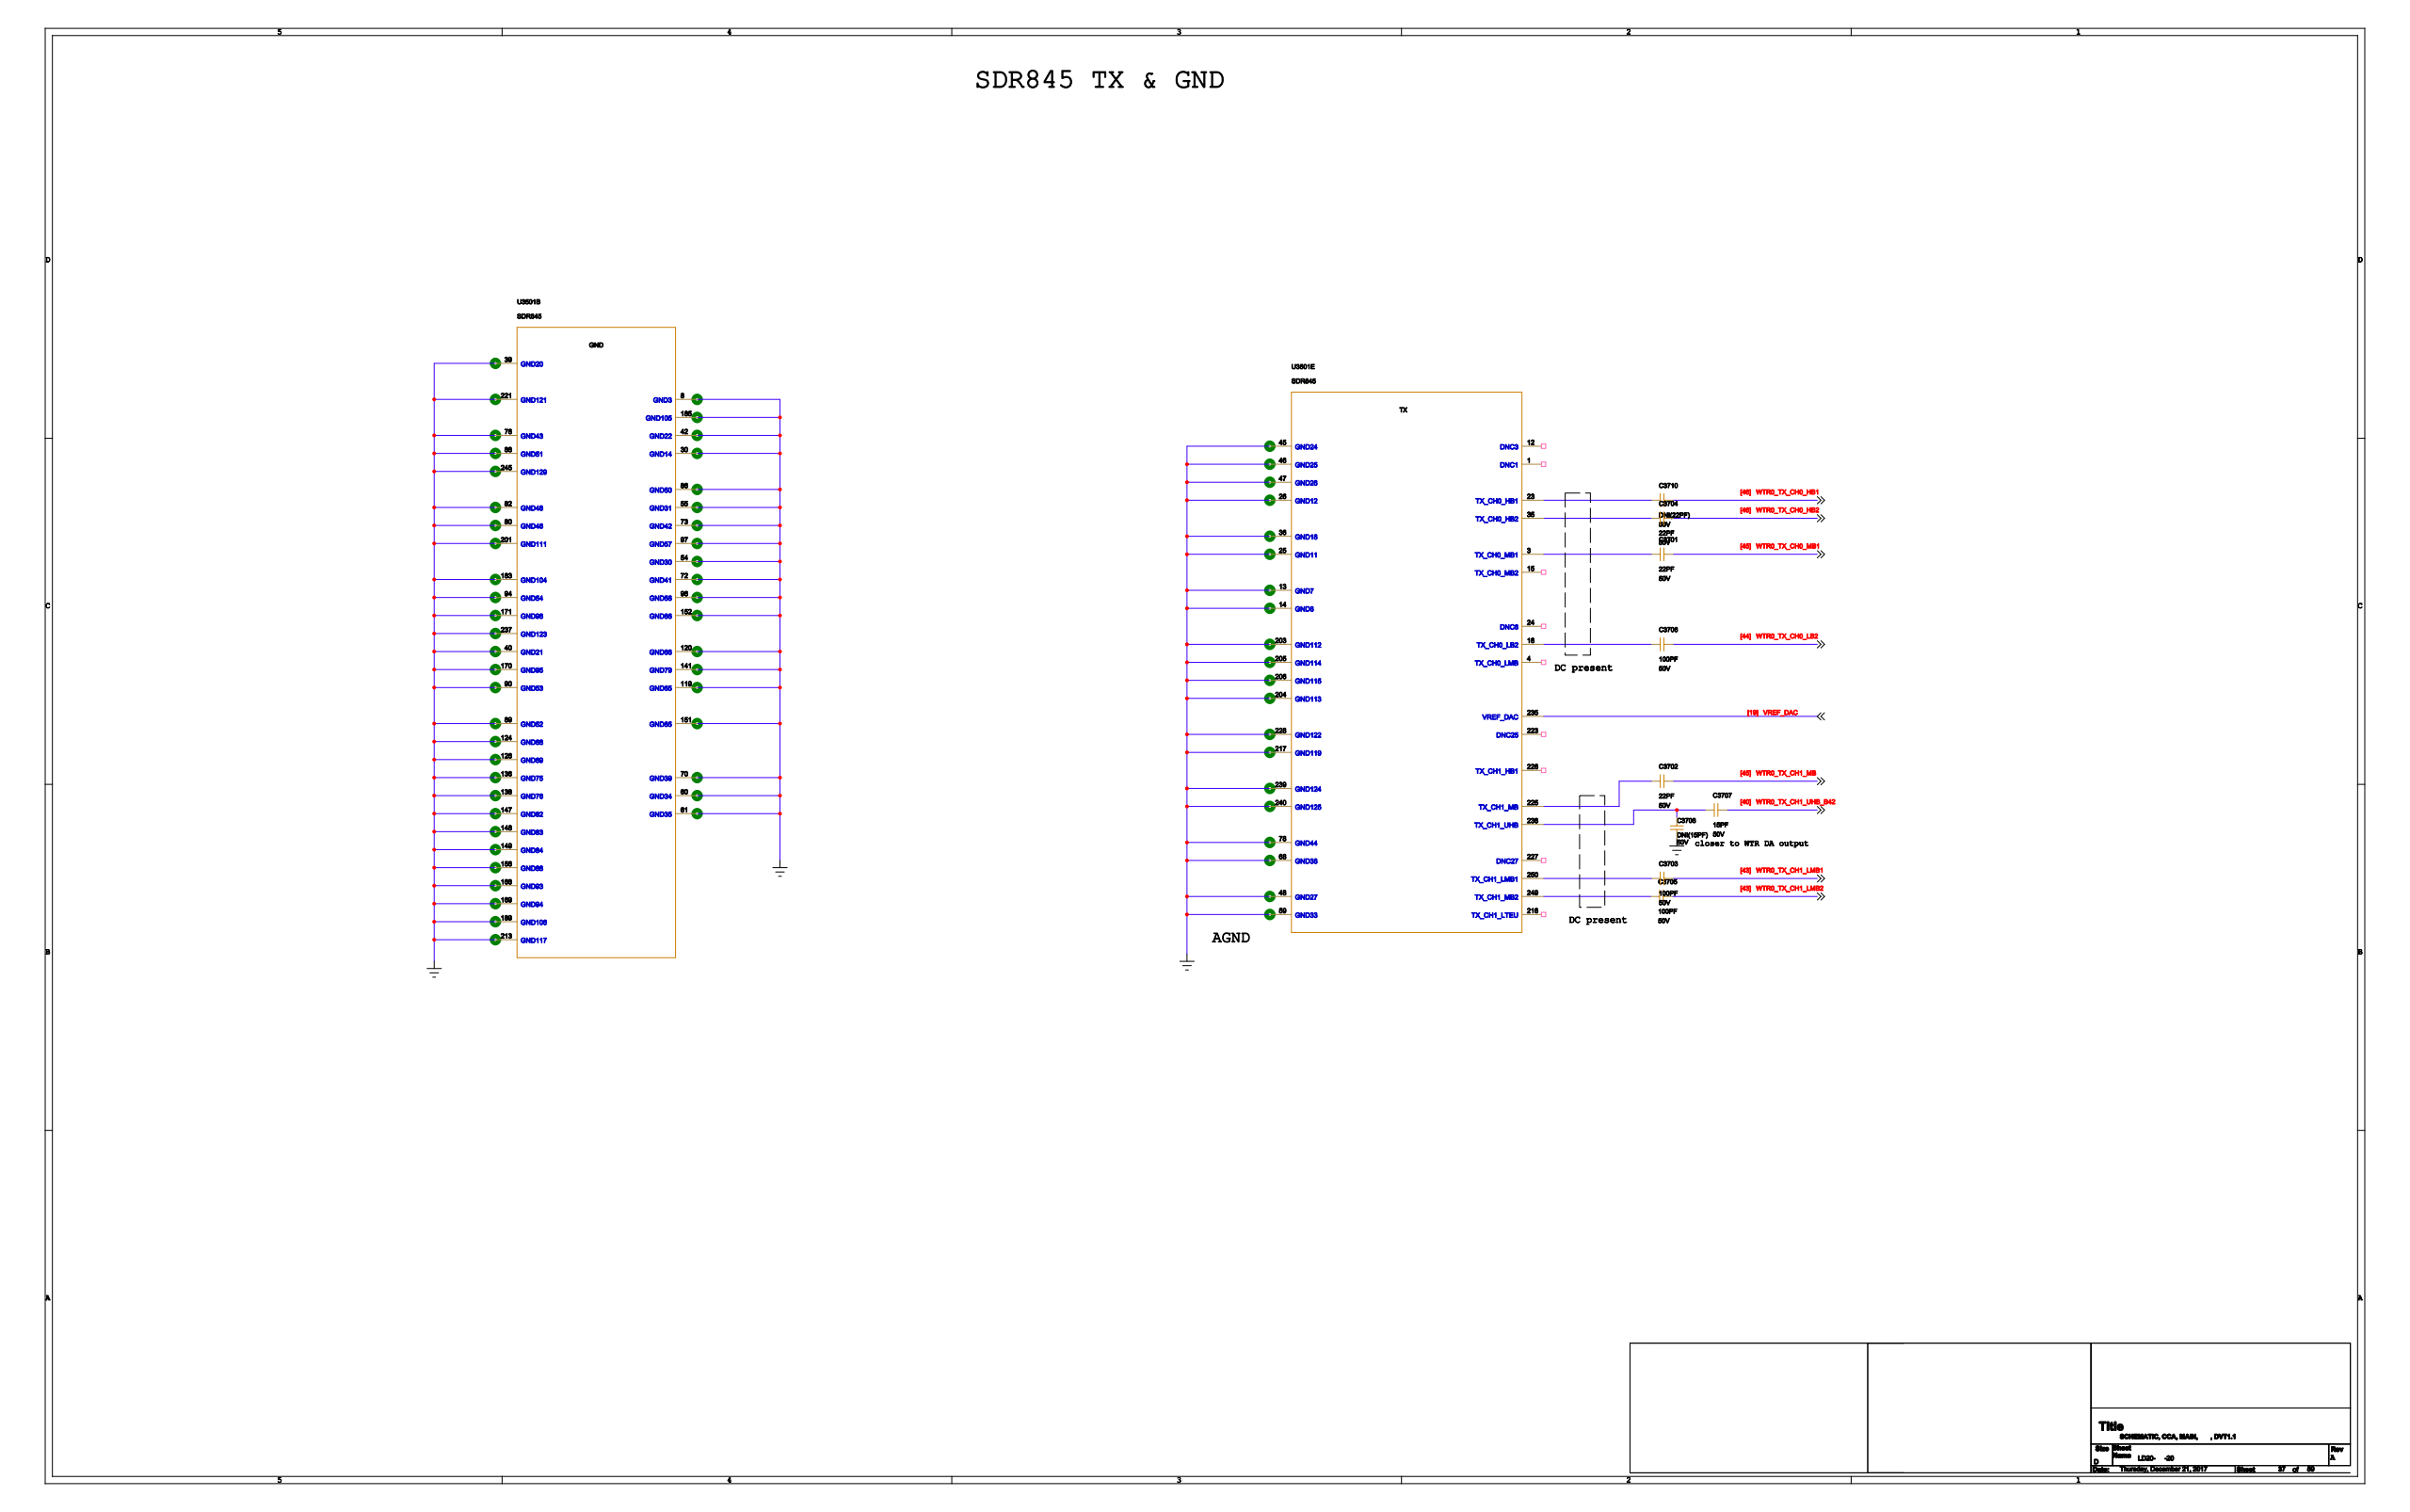Circuit board | Cadence Allegro | 1520 parts | 1149 nets | one sheet of the schematic
Parts on this sheet (reference | value | footprint):
C3701 | 22PF | 2P0201R
C3702 | 22PF | 2P0201R
C3703 | 100PF | 2P0201R
C3704 | 22PF | 2P0201R
C3705 | 100PF | 2P0201R
C3706 | 100PF | 2P0201R
C3707 | 15PF | 2P0201R
C3708 | DNI(15PF) | 2P0201R_DNI
C3710 | DNI(22PF) | 2P0201R_DNI
U3501 | SDR845 | 253PGA235X247B138D45
Nets of these parts (net: part-pin ...):
N48224363: C3707-1 C3708-1 U3501-238
GND: C3708-2 U3501-8 U3501-11 U3501-13 U3501-14 U3501-21 U3501-22 U3501-25 U3501-26 U3501-30 U3501-33 U3501-36 U3501-39 U3501-40 U3501-42 U3501-45 U3501-46 U3501-47 U3501-48 U3501-54 U3501-55 U3501-59 U3501-60 U3501-61 U3501-68 U3501-70 U3501-72 U3501-73 U3501-76 U3501-78 U3501-80 U3501-82 U3501-86 U3501-88 U3501-89 U3501-90 U3501-94 U3501-96 U3501-97 U3501-119 U3501-120 U3501-124 U3501-126 U3501-136 U3501-138 U3501-141 U3501-147 U3501-148 U3501-149 U3501-151 U3501-152 U3501-156 U3501-168 U3501-169 U3501-170 U3501-171 U3501-183 U3501-185 U3501-189 U3501-201 U3501-203 U3501-204 U3501-205 U3501-206 U3501-213 U3501-217 U3501-221 U3501-228 U3501-237 U3501-239 U3501-240 U3501-245
WTR0_TX_CH1_UHB_B42: C3707-2
N49033316: C3710-1 U3501-23
WTR0_TX_CH0_HB1: C3710-2
N35858069: C3704-1 U3501-35
N48051304: C3706-1 U3501-16
N48051262: C3701-1 U3501-3
N48051430: C3703-1 U3501-250
N48223922: C3702-1 U3501-225
N48051470: C3705-1 U3501-249
VREF_DAC: U3501-235
WTR0_TX_CH0_MB1: C3701-2
WTR0_TX_CH1_MB: C3702-2
WTR0_TX_CH0_HB2: C3704-2
WTR0_TX_CH0_LB2: C3706-2
WTR0_TX_CH1_LMB1: C3703-2
WTR0_TX_CH1_LMB2: C3705-2